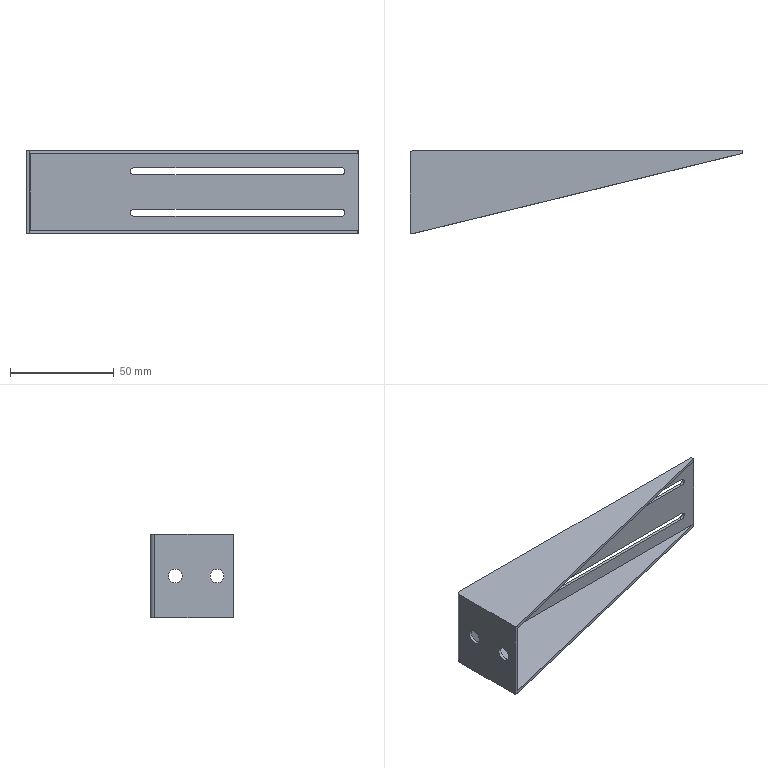Part | NX | 1 solid | 24 faces | box 160 x 40 x 40 mm | volume 19881 mm3 | plane 16 | cylinder 8 | commonest cylinder face diameters 3.4 x4 6.6 x2 1 x1 4 x1
STEP:
#1=CARTESIAN_POINT('',(159.99,-1.5,-18.5));
#2=VERTEX_POINT('',#1);
#3=CARTESIAN_POINT('',(2.,-1.5,-18.5));
#4=VERTEX_POINT('',#3);
#5=CARTESIAN_POINT('',(0.,-1.5,-18.5));
#6=DIRECTION('',(-1.,0.,0.));
#7=VECTOR('',#6,1000.);
#8=LINE('',#5,#7);
#9=EDGE_CURVE('',#2,#4,#8,.T.);
#10=ORIENTED_EDGE('',*,*,#9,.F.);
#11=CARTESIAN_POINT('',(159.99,-1.5,-20.));
#12=VERTEX_POINT('',#11);
#13=CARTESIAN_POINT('',(159.99,-1.5,20.));
#14=DIRECTION('',(0.,0.,1.));
#15=VECTOR('',#14,1000.);
#16=LINE('',#13,#15);
#17=EDGE_CURVE('',#2,#12,#16,.F.);
#18=ORIENTED_EDGE('',*,*,#17,.T.);
#19=CARTESIAN_POINT('',(160.,-1.5,-20.));
#20=VERTEX_POINT('',#19);
#21=CARTESIAN_POINT('',(0.,-1.5,-20.));
#22=DIRECTION('',(1.,0.,0.));
#23=VECTOR('',#22,1000.);
#24=LINE('',#21,#23);
#25=EDGE_CURVE('',#12,#20,#24,.T.);
#26=ORIENTED_EDGE('',*,*,#25,.T.);
#27=CARTESIAN_POINT('',(160.,-1.5,20.));
#28=VERTEX_POINT('',#27);
#29=CARTESIAN_POINT('',(160.,-1.5,20.));
#30=DIRECTION('',(0.,0.,-1.));
#31=VECTOR('',#30,1000.);
#32=LINE('',#29,#31);
#33=EDGE_CURVE('',#28,#20,#32,.T.);
#34=ORIENTED_EDGE('',*,*,#33,.F.);
#35=CARTESIAN_POINT('',(159.99,-1.5,20.));
#36=VERTEX_POINT('',#35);
#37=CARTESIAN_POINT('',(0.,-1.5,20.));
#38=DIRECTION('',(1.,0.,0.));
#39=VECTOR('',#38,1000.);
#40=LINE('',#37,#39);
#41=EDGE_CURVE('',#36,#28,#40,.T.);
#42=ORIENTED_EDGE('',*,*,#41,.F.);
#43=CARTESIAN_POINT('',(159.99,-1.5,18.5));
#44=VERTEX_POINT('',#43);
#45=CARTESIAN_POINT('',(159.99,-1.5,20.));
#46=DIRECTION('',(0.,0.,-1.));
#47=VECTOR('',#46,1000.);
#48=LINE('',#45,#47);
#49=EDGE_CURVE('',#36,#44,#48,.T.);
#50=ORIENTED_EDGE('',*,*,#49,.T.);
#51=CARTESIAN_POINT('',(2.,-1.5,18.5));
#52=VERTEX_POINT('',#51);
#53=CARTESIAN_POINT('',(0.,-1.5,18.5));
#54=DIRECTION('',(1.,0.,0.));
#55=VECTOR('',#54,1000.);
#56=LINE('',#53,#55);
#57=EDGE_CURVE('',#52,#44,#56,.T.);
#58=ORIENTED_EDGE('',*,*,#57,.F.);
#59=CARTESIAN_POINT('',(2.,-1.5,20.));
#60=DIRECTION('',(0.,0.,-1.));
#61=VECTOR('',#60,1000.);
#62=LINE('',#59,#61);
#63=EDGE_CURVE('',#52,#4,#62,.T.);
#64=ORIENTED_EDGE('',*,*,#63,.T.);
#65=EDGE_LOOP('',(#10,#18,#26,#34,#42,#50,#58,#64));
#66=FACE_BOUND('',#65,.T.);
#67=CARTESIAN_POINT('',(152.,-1.5,8.3));
#68=VERTEX_POINT('',#67);
#69=CARTESIAN_POINT('',(52.,-1.5,8.3));
#70=VERTEX_POINT('',#69);
#71=CARTESIAN_POINT('',(52.,-1.5,8.3));
#72=DIRECTION('',(-1.,0.,0.));
#73=VECTOR('',#72,1000.);
#74=LINE('',#71,#73);
#75=EDGE_CURVE('',#68,#70,#74,.T.);
#76=ORIENTED_EDGE('',*,*,#75,.T.);
#77=CARTESIAN_POINT('',(52.,-1.5,11.7));
#78=VERTEX_POINT('',#77);
#79=CARTESIAN_POINT('',(52.,-1.5,10.));
#80=DIRECTION('',(0.,1.,0.));
#81=DIRECTION('',(0.,0.,1.));
#82=AXIS2_PLACEMENT_3D('',#79,#80,#81);
#83=CIRCLE('',#82,1.7);
#84=EDGE_CURVE('',#70,#78,#83,.T.);
#85=ORIENTED_EDGE('',*,*,#84,.T.);
#86=CARTESIAN_POINT('',(152.,-1.5,11.7));
#87=VERTEX_POINT('',#86);
#88=CARTESIAN_POINT('',(52.,-1.5,11.7));
#89=DIRECTION('',(1.,0.,0.));
#90=VECTOR('',#89,1000.);
#91=LINE('',#88,#90);
#92=EDGE_CURVE('',#78,#87,#91,.T.);
#93=ORIENTED_EDGE('',*,*,#92,.T.);
#94=CARTESIAN_POINT('',(152.,-1.5,10.));
#95=DIRECTION('',(0.,1.,0.));
#96=DIRECTION('',(0.,0.,1.));
#97=AXIS2_PLACEMENT_3D('',#94,#95,#96);
#98=CIRCLE('',#97,1.7);
#99=EDGE_CURVE('',#87,#68,#98,.T.);
#100=ORIENTED_EDGE('',*,*,#99,.T.);
#101=EDGE_LOOP('',(#76,#85,#93,#100));
#102=FACE_BOUND('',#101,.T.);
#103=CARTESIAN_POINT('',(52.,-1.5,-8.3));
#104=VERTEX_POINT('',#103);
#105=CARTESIAN_POINT('',(52.,-1.5,-11.7));
#106=VERTEX_POINT('',#105);
#107=CARTESIAN_POINT('',(52.,-1.5,-10.));
#108=DIRECTION('',(0.,-1.,0.));
#109=DIRECTION('',(0.,0.,-1.));
#110=AXIS2_PLACEMENT_3D('',#107,#108,#109);
#111=CIRCLE('',#110,1.7);
#112=EDGE_CURVE('',#104,#106,#111,.T.);
#113=ORIENTED_EDGE('',*,*,#112,.F.);
#114=CARTESIAN_POINT('',(152.,-1.5,-8.3));
#115=VERTEX_POINT('',#114);
#116=CARTESIAN_POINT('',(52.,-1.5,-8.3));
#117=DIRECTION('',(-1.,0.,0.));
#118=VECTOR('',#117,1000.);
#119=LINE('',#116,#118);
#120=EDGE_CURVE('',#115,#104,#119,.T.);
#121=ORIENTED_EDGE('',*,*,#120,.F.);
#122=CARTESIAN_POINT('',(152.,-1.5,-11.7));
#123=VERTEX_POINT('',#122);
#124=CARTESIAN_POINT('',(152.,-1.5,-10.));
#125=DIRECTION('',(0.,-1.,0.));
#126=DIRECTION('',(0.,0.,-1.));
#127=AXIS2_PLACEMENT_3D('',#124,#125,#126);
#128=CIRCLE('',#127,1.7);
#129=EDGE_CURVE('',#123,#115,#128,.T.);
#130=ORIENTED_EDGE('',*,*,#129,.F.);
#131=CARTESIAN_POINT('',(52.,-1.5,-11.7));
#132=DIRECTION('',(1.,0.,0.));
#133=VECTOR('',#132,1000.);
#134=LINE('',#131,#133);
#135=EDGE_CURVE('',#106,#123,#134,.T.);
#136=ORIENTED_EDGE('',*,*,#135,.F.);
#137=EDGE_LOOP('',(#113,#121,#130,#136));
#138=FACE_BOUND('',#137,.T.);
#139=CARTESIAN_POINT('',(0.,-1.5,20.));
#140=DIRECTION('',(0.,1.,0.));
#141=DIRECTION('',(0.,0.,1.));
#142=AXIS2_PLACEMENT_3D('',#139,#140,#141);
#143=PLANE('',#142);
#144=ADVANCED_FACE('',(#66,#102,#138),#143,.F.);
#145=CARTESIAN_POINT('',(52.,0.,8.3));
#146=VERTEX_POINT('',#145);
#147=CARTESIAN_POINT('',(52.,0.,11.7));
#148=VERTEX_POINT('',#147);
#149=CARTESIAN_POINT('',(52.,0.,10.));
#150=DIRECTION('',(0.,1.,0.));
#151=DIRECTION('',(0.,0.,1.));
#152=AXIS2_PLACEMENT_3D('',#149,#150,#151);
#153=CIRCLE('',#152,1.7);
#154=EDGE_CURVE('',#146,#148,#153,.T.);
#155=ORIENTED_EDGE('',*,*,#154,.F.);
#156=CARTESIAN_POINT('',(152.,0.,8.3));
#157=VERTEX_POINT('',#156);
#158=CARTESIAN_POINT('',(52.,0.,8.3));
#159=DIRECTION('',(-1.,0.,0.));
#160=VECTOR('',#159,1000.);
#161=LINE('',#158,#160);
#162=EDGE_CURVE('',#157,#146,#161,.T.);
#163=ORIENTED_EDGE('',*,*,#162,.F.);
#164=CARTESIAN_POINT('',(152.,0.,11.7));
#165=VERTEX_POINT('',#164);
#166=CARTESIAN_POINT('',(152.,0.,10.));
#167=DIRECTION('',(0.,1.,0.));
#168=DIRECTION('',(0.,0.,1.));
#169=AXIS2_PLACEMENT_3D('',#166,#167,#168);
#170=CIRCLE('',#169,1.7);
#171=EDGE_CURVE('',#165,#157,#170,.T.);
#172=ORIENTED_EDGE('',*,*,#171,.F.);
#173=CARTESIAN_POINT('',(52.,0.,11.7));
#174=DIRECTION('',(1.,0.,0.));
#175=VECTOR('',#174,1000.);
#176=LINE('',#173,#175);
#177=EDGE_CURVE('',#148,#165,#176,.T.);
#178=ORIENTED_EDGE('',*,*,#177,.F.);
#179=EDGE_LOOP('',(#155,#163,#172,#178));
#180=FACE_BOUND('',#179,.T.);
#181=CARTESIAN_POINT('',(2.,0.,-20.));
#182=VERTEX_POINT('',#181);
#183=CARTESIAN_POINT('',(160.,0.,-20.));
#184=VERTEX_POINT('',#183);
#185=CARTESIAN_POINT('',(0.,0.,-20.));
#186=DIRECTION('',(1.,0.,0.));
#187=VECTOR('',#186,1000.);
#188=LINE('',#185,#187);
#189=EDGE_CURVE('',#182,#184,#188,.T.);
#190=ORIENTED_EDGE('',*,*,#189,.F.);
#191=CARTESIAN_POINT('',(2.,0.,20.));
#192=VERTEX_POINT('',#191);
#193=CARTESIAN_POINT('',(2.,0.,20.));
#194=DIRECTION('',(0.,0.,-1.));
#195=VECTOR('',#194,1000.);
#196=LINE('',#193,#195);
#197=EDGE_CURVE('',#192,#182,#196,.T.);
#198=ORIENTED_EDGE('',*,*,#197,.F.);
#199=CARTESIAN_POINT('',(160.,0.,20.));
#200=VERTEX_POINT('',#199);
#201=CARTESIAN_POINT('',(0.,0.,20.));
#202=DIRECTION('',(1.,0.,0.));
#203=VECTOR('',#202,1000.);
#204=LINE('',#201,#203);
#205=EDGE_CURVE('',#192,#200,#204,.T.);
#206=ORIENTED_EDGE('',*,*,#205,.T.);
#207=CARTESIAN_POINT('',(160.,0.,20.));
#208=DIRECTION('',(0.,0.,-1.));
#209=VECTOR('',#208,1000.);
#210=LINE('',#207,#209);
#211=EDGE_CURVE('',#200,#184,#210,.T.);
#212=ORIENTED_EDGE('',*,*,#211,.T.);
#213=EDGE_LOOP('',(#190,#198,#206,#212));
#214=FACE_BOUND('',#213,.T.);
#215=CARTESIAN_POINT('',(152.,0.,-8.3));
#216=VERTEX_POINT('',#215);
#217=CARTESIAN_POINT('',(52.,0.,-8.3));
#218=VERTEX_POINT('',#217);
#219=CARTESIAN_POINT('',(52.,0.,-8.3));
#220=DIRECTION('',(-1.,0.,0.));
#221=VECTOR('',#220,1000.);
#222=LINE('',#219,#221);
#223=EDGE_CURVE('',#216,#218,#222,.T.);
#224=ORIENTED_EDGE('',*,*,#223,.T.);
#225=CARTESIAN_POINT('',(52.,0.,-11.7));
#226=VERTEX_POINT('',#225);
#227=CARTESIAN_POINT('',(52.,0.,-10.));
#228=DIRECTION('',(0.,-1.,0.));
#229=DIRECTION('',(0.,0.,-1.));
#230=AXIS2_PLACEMENT_3D('',#227,#228,#229);
#231=CIRCLE('',#230,1.7);
#232=EDGE_CURVE('',#218,#226,#231,.T.);
#233=ORIENTED_EDGE('',*,*,#232,.T.);
#234=CARTESIAN_POINT('',(152.,0.,-11.7));
#235=VERTEX_POINT('',#234);
#236=CARTESIAN_POINT('',(52.,0.,-11.7));
#237=DIRECTION('',(1.,0.,0.));
#238=VECTOR('',#237,1000.);
#239=LINE('',#236,#238);
#240=EDGE_CURVE('',#226,#235,#239,.T.);
#241=ORIENTED_EDGE('',*,*,#240,.T.);
#242=CARTESIAN_POINT('',(152.,0.,-10.));
#243=DIRECTION('',(0.,-1.,0.));
#244=DIRECTION('',(0.,0.,-1.));
#245=AXIS2_PLACEMENT_3D('',#242,#243,#244);
#246=CIRCLE('',#245,1.7);
#247=EDGE_CURVE('',#235,#216,#246,.T.);
#248=ORIENTED_EDGE('',*,*,#247,.T.);
#249=EDGE_LOOP('',(#224,#233,#241,#248));
#250=FACE_BOUND('',#249,.T.);
#251=CARTESIAN_POINT('',(0.,0.,20.));
#252=DIRECTION('',(0.,1.,0.));
#253=DIRECTION('',(0.,0.,1.));
#254=AXIS2_PLACEMENT_3D('',#251,#252,#253);
#255=PLANE('',#254);
#256=ADVANCED_FACE('',(#180,#214,#250),#255,.T.);
#257=CARTESIAN_POINT('',(1.5,-12.,3.3));
#258=VERTEX_POINT('',#257);
#259=CARTESIAN_POINT('',(1.5,-12.,0.));
#260=DIRECTION('',(-1.,0.,0.));
#261=DIRECTION('',(0.,0.,1.));
#262=AXIS2_PLACEMENT_3D('',#259,#260,#261);
#263=CIRCLE('',#262,3.3);
#264=EDGE_CURVE('',#258,#258,#263,.T.);
#265=ORIENTED_EDGE('',*,*,#264,.T.);
#266=EDGE_LOOP('',(#265));
#267=FACE_BOUND('',#266,.T.);
#268=CARTESIAN_POINT('',(1.5,-32.,3.3));
#269=VERTEX_POINT('',#268);
#270=CARTESIAN_POINT('',(1.5,-32.,0.));
#271=DIRECTION('',(-1.,0.,0.));
#272=DIRECTION('',(0.,0.,1.));
#273=AXIS2_PLACEMENT_3D('',#270,#271,#272);
#274=CIRCLE('',#273,3.3);
#275=EDGE_CURVE('',#269,#269,#274,.T.);
#276=ORIENTED_EDGE('',*,*,#275,.T.);
#277=EDGE_LOOP('',(#276));
#278=FACE_BOUND('',#277,.T.);
#279=CARTESIAN_POINT('',(1.5,-2.,-18.5));
#280=VERTEX_POINT('',#279);
#281=CARTESIAN_POINT('',(1.5,-40.,-18.5));
#282=VERTEX_POINT('',#281);
#283=CARTESIAN_POINT('',(1.5,-40.,-18.5));
#284=DIRECTION('',(0.,-1.,0.));
#285=VECTOR('',#284,1000.);
#286=LINE('',#283,#285);
#287=EDGE_CURVE('',#280,#282,#286,.T.);
#288=ORIENTED_EDGE('',*,*,#287,.F.);
#289=CARTESIAN_POINT('',(1.5,-2.,18.5));
#290=VERTEX_POINT('',#289);
#291=CARTESIAN_POINT('',(1.5,-2.,20.));
#292=DIRECTION('',(0.,0.,-1.));
#293=VECTOR('',#292,1000.);
#294=LINE('',#291,#293);
#295=EDGE_CURVE('',#290,#280,#294,.T.);
#296=ORIENTED_EDGE('',*,*,#295,.F.);
#297=CARTESIAN_POINT('',(1.5,-40.,18.5));
#298=VERTEX_POINT('',#297);
#299=CARTESIAN_POINT('',(1.5,-40.,18.5));
#300=DIRECTION('',(0.,1.,0.));
#301=VECTOR('',#300,1000.);
#302=LINE('',#299,#301);
#303=EDGE_CURVE('',#298,#290,#302,.T.);
#304=ORIENTED_EDGE('',*,*,#303,.F.);
#305=CARTESIAN_POINT('',(1.5,-40.,20.));
#306=DIRECTION('',(0.,0.,-1.));
#307=VECTOR('',#306,1000.);
#308=LINE('',#305,#307);
#309=EDGE_CURVE('',#298,#282,#308,.T.);
#310=ORIENTED_EDGE('',*,*,#309,.T.);
#311=EDGE_LOOP('',(#288,#296,#304,#310));
#312=FACE_BOUND('',#311,.T.);
#313=CARTESIAN_POINT('',(1.5,-40.,20.));
#314=DIRECTION('',(-1.,0.,0.));
#315=DIRECTION('',(0.,0.,1.));
#316=AXIS2_PLACEMENT_3D('',#313,#314,#315);
#317=PLANE('',#316);
#318=ADVANCED_FACE('',(#267,#278,#312),#317,.F.);
#319=CARTESIAN_POINT('',(2.,-2.,-18.5));
#320=DIRECTION('',(0.,0.,-1.));
#321=DIRECTION('',(-1.,0.,0.));
#322=AXIS2_PLACEMENT_3D('',#319,#320,#321);
#323=CIRCLE('',#322,0.5);
#324=EDGE_CURVE('',#4,#280,#323,.F.);
#325=ORIENTED_EDGE('',*,*,#324,.F.);
#326=ORIENTED_EDGE('',*,*,#63,.F.);
#327=CARTESIAN_POINT('',(2.,-2.,18.5));
#328=DIRECTION('',(0.,0.,1.));
#329=DIRECTION('',(1.,0.,0.));
#330=AXIS2_PLACEMENT_3D('',#327,#328,#329);
#331=CIRCLE('',#330,0.5);
#332=EDGE_CURVE('',#290,#52,#331,.F.);
#333=ORIENTED_EDGE('',*,*,#332,.F.);
#334=ORIENTED_EDGE('',*,*,#295,.T.);
#335=EDGE_LOOP('',(#325,#326,#333,#334));
#336=FACE_BOUND('',#335,.T.);
#337=CARTESIAN_POINT('',(2.,-2.,20.));
#338=DIRECTION('',(0.,0.,-1.));
#339=DIRECTION('',(-1.,0.,0.));
#340=AXIS2_PLACEMENT_3D('',#337,#338,#339);
#341=CYLINDRICAL_SURFACE('',#340,0.5);
#342=ADVANCED_FACE('',(#336),#341,.F.);
#343=ORIENTED_EDGE('',*,*,#33,.T.);
#344=CARTESIAN_POINT('',(160.,0.,-20.));
#345=DIRECTION('',(0.,-1.,0.));
#346=VECTOR('',#345,1000.);
#347=LINE('',#344,#346);
#348=EDGE_CURVE('',#184,#20,#347,.T.);
#349=ORIENTED_EDGE('',*,*,#348,.F.);
#350=ORIENTED_EDGE('',*,*,#211,.F.);
#351=CARTESIAN_POINT('',(160.,0.,20.));
#352=DIRECTION('',(0.,-1.,0.));
#353=VECTOR('',#352,1000.);
#354=LINE('',#351,#353);
#355=EDGE_CURVE('',#200,#28,#354,.T.);
#356=ORIENTED_EDGE('',*,*,#355,.T.);
#357=EDGE_LOOP('',(#343,#349,#350,#356));
#358=FACE_BOUND('',#357,.T.);
#359=CARTESIAN_POINT('',(160.,0.,20.));
#360=DIRECTION('',(1.,0.,0.));
#361=DIRECTION('',(0.,0.,-1.));
#362=AXIS2_PLACEMENT_3D('',#359,#360,#361);
#363=PLANE('',#362);
#364=ADVANCED_FACE('',(#358),#363,.T.);
#365=CARTESIAN_POINT('',(0.,-2.,-20.));
#366=VERTEX_POINT('',#365);
#367=CARTESIAN_POINT('',(2.,-2.,-20.));
#368=DIRECTION('',(0.,0.,1.));
#369=DIRECTION('',(1.,0.,0.));
#370=AXIS2_PLACEMENT_3D('',#367,#368,#369);
#371=CIRCLE('',#370,2.);
#372=EDGE_CURVE('',#366,#182,#371,.F.);
#373=ORIENTED_EDGE('',*,*,#372,.F.);
#374=CARTESIAN_POINT('',(0.,-2.,20.));
#375=VERTEX_POINT('',#374);
#376=CARTESIAN_POINT('',(0.,-2.,20.));
#377=DIRECTION('',(0.,0.,-1.));
#378=VECTOR('',#377,1000.);
#379=LINE('',#376,#378);
#380=EDGE_CURVE('',#375,#366,#379,.T.);
#381=ORIENTED_EDGE('',*,*,#380,.F.);
#382=CARTESIAN_POINT('',(2.,-2.,20.));
#383=DIRECTION('',(0.,0.,1.));
#384=DIRECTION('',(1.,0.,0.));
#385=AXIS2_PLACEMENT_3D('',#382,#383,#384);
#386=CIRCLE('',#385,2.);
#387=EDGE_CURVE('',#375,#192,#386,.F.);
#388=ORIENTED_EDGE('',*,*,#387,.T.);
#389=ORIENTED_EDGE('',*,*,#197,.T.);
#390=EDGE_LOOP('',(#373,#381,#388,#389));
#391=FACE_BOUND('',#390,.T.);
#392=CARTESIAN_POINT('',(2.,-2.,20.));
#393=DIRECTION('',(0.,0.,-1.));
#394=DIRECTION('',(-1.,0.,0.));
#395=AXIS2_PLACEMENT_3D('',#392,#393,#394);
#396=CYLINDRICAL_SURFACE('',#395,2.);
#397=ADVANCED_FACE('',(#391),#396,.T.);
#398=CARTESIAN_POINT('',(0.,-12.,3.3));
#399=VERTEX_POINT('',#398);
#400=CARTESIAN_POINT('',(0.,-12.,0.));
#401=DIRECTION('',(-1.,0.,0.));
#402=DIRECTION('',(0.,0.,1.));
#403=AXIS2_PLACEMENT_3D('',#400,#401,#402);
#404=CIRCLE('',#403,3.3);
#405=EDGE_CURVE('',#399,#399,#404,.T.);
#406=ORIENTED_EDGE('',*,*,#405,.F.);
#407=EDGE_LOOP('',(#406));
#408=FACE_BOUND('',#407,.T.);
#409=CARTESIAN_POINT('',(0.,-32.,3.3));
#410=VERTEX_POINT('',#409);
#411=CARTESIAN_POINT('',(0.,-32.,0.));
#412=DIRECTION('',(-1.,0.,0.));
#413=DIRECTION('',(0.,0.,1.));
#414=AXIS2_PLACEMENT_3D('',#411,#412,#413);
#415=CIRCLE('',#414,3.3);
#416=EDGE_CURVE('',#410,#410,#415,.T.);
#417=ORIENTED_EDGE('',*,*,#416,.F.);
#418=EDGE_LOOP('',(#417));
#419=FACE_BOUND('',#418,.T.);
#420=CARTESIAN_POINT('',(0.,-40.,-20.));
#421=VERTEX_POINT('',#420);
#422=CARTESIAN_POINT('',(0.,-40.,-20.));
#423=DIRECTION('',(0.,1.,0.));
#424=VECTOR('',#423,1000.);
#425=LINE('',#422,#424);
#426=EDGE_CURVE('',#421,#366,#425,.T.);
#427=ORIENTED_EDGE('',*,*,#426,.F.);
#428=CARTESIAN_POINT('',(0.,-40.,20.));
#429=VERTEX_POINT('',#428);
#430=CARTESIAN_POINT('',(0.,-40.,20.));
#431=DIRECTION('',(0.,0.,-1.));
#432=VECTOR('',#431,1000.);
#433=LINE('',#430,#432);
#434=EDGE_CURVE('',#429,#421,#433,.T.);
#435=ORIENTED_EDGE('',*,*,#434,.F.);
#436=CARTESIAN_POINT('',(0.,-40.,20.));
#437=DIRECTION('',(0.,1.,0.));
#438=VECTOR('',#437,1000.);
#439=LINE('',#436,#438);
#440=EDGE_CURVE('',#429,#375,#439,.T.);
#441=ORIENTED_EDGE('',*,*,#440,.T.);
#442=ORIENTED_EDGE('',*,*,#380,.T.);
#443=EDGE_LOOP('',(#427,#435,#441,#442));
#444=FACE_BOUND('',#443,.T.);
#445=CARTESIAN_POINT('',(0.,-40.,20.));
#446=DIRECTION('',(-1.,0.,0.));
#447=DIRECTION('',(0.,0.,1.));
#448=AXIS2_PLACEMENT_3D('',#445,#446,#447);
#449=PLANE('',#448);
#450=ADVANCED_FACE('',(#408,#419,#444),#449,.T.);
#451=CARTESIAN_POINT('',(1.5,-40.,-20.));
#452=VERTEX_POINT('',#451);
#453=CARTESIAN_POINT('',(1.5,-40.,20.));
#454=DIRECTION('',(0.,0.,-1.));
#455=VECTOR('',#454,1000.);
#456=LINE('',#453,#455);
#457=EDGE_CURVE('',#452,#282,#456,.F.);
#458=ORIENTED_EDGE('',*,*,#457,.T.);
#459=ORIENTED_EDGE('',*,*,#309,.F.);
#460=CARTESIAN_POINT('',(1.5,-40.,20.));
#461=VERTEX_POINT('',#460);
#462=CARTESIAN_POINT('',(1.5,-40.,20.));
#463=DIRECTION('',(0.,0.,-1.));
#464=VECTOR('',#463,1000.);
#465=LINE('',#462,#464);
#466=EDGE_CURVE('',#461,#298,#465,.T.);
#467=ORIENTED_EDGE('',*,*,#466,.F.);
#468=CARTESIAN_POINT('',(1.5,-40.,20.));
#469=DIRECTION('',(-1.,0.,0.));
#470=VECTOR('',#469,1000.);
#471=LINE('',#468,#470);
#472=EDGE_CURVE('',#461,#429,#471,.T.);
#473=ORIENTED_EDGE('',*,*,#472,.T.);
#474=ORIENTED_EDGE('',*,*,#434,.T.);
#475=CARTESIAN_POINT('',(1.5,-40.,-20.));
#476=DIRECTION('',(-1.,0.,0.));
#477=VECTOR('',#476,1000.);
#478=LINE('',#475,#477);
#479=EDGE_CURVE('',#452,#421,#478,.T.);
#480=ORIENTED_EDGE('',*,*,#479,.F.);
#481=EDGE_LOOP('',(#458,#459,#467,#473,#474,#480));
#482=FACE_BOUND('',#481,.T.);
#483=CARTESIAN_POINT('',(1.5,-40.,20.));
#484=DIRECTION('',(0.,-1.,0.));
#485=DIRECTION('',(0.,0.,-1.));
#486=AXIS2_PLACEMENT_3D('',#483,#484,#485);
#487=PLANE('',#486);
#488=ADVANCED_FACE('',(#482),#487,.T.);
#489=CARTESIAN_POINT('',(1.5,-40.,20.));
#490=DIRECTION('',(0.9717,0.2361,0.));
#491=VECTOR('',#490,1000.);
#492=LINE('',#489,#491);
#493=EDGE_CURVE('',#461,#36,#492,.T.);
#494=ORIENTED_EDGE('',*,*,#493,.T.);
#495=ORIENTED_EDGE('',*,*,#41,.T.);
#496=ORIENTED_EDGE('',*,*,#355,.F.);
#497=ORIENTED_EDGE('',*,*,#205,.F.);
#498=ORIENTED_EDGE('',*,*,#387,.F.);
#499=ORIENTED_EDGE('',*,*,#440,.F.);
#500=ORIENTED_EDGE('',*,*,#472,.F.);
#501=EDGE_LOOP('',(#494,#495,#496,#497,#498,#499,#500));
#502=FACE_BOUND('',#501,.T.);
#503=CARTESIAN_POINT('',(2.,-2.,20.));
#504=DIRECTION('',(0.,0.,1.));
#505=DIRECTION('',(1.,0.,0.));
#506=AXIS2_PLACEMENT_3D('',#503,#504,#505);
#507=PLANE('',#506);
#508=ADVANCED_FACE('',(#502),#507,.T.);
#509=ORIENTED_EDGE('',*,*,#25,.F.);
#510=CARTESIAN_POINT('',(1.5,-40.,-20.));
#511=DIRECTION('',(0.9717,0.2361,0.));
#512=VECTOR('',#511,1000.);
#513=LINE('',#510,#512);
#514=EDGE_CURVE('',#452,#12,#513,.T.);
#515=ORIENTED_EDGE('',*,*,#514,.F.);
#516=ORIENTED_EDGE('',*,*,#479,.T.);
#517=ORIENTED_EDGE('',*,*,#426,.T.);
#518=ORIENTED_EDGE('',*,*,#372,.T.);
#519=ORIENTED_EDGE('',*,*,#189,.T.);
#520=ORIENTED_EDGE('',*,*,#348,.T.);
#521=EDGE_LOOP('',(#509,#515,#516,#517,#518,#519,#520));
#522=FACE_BOUND('',#521,.T.);
#523=CARTESIAN_POINT('',(2.,-2.,-20.));
#524=DIRECTION('',(0.,0.,1.));
#525=DIRECTION('',(1.,0.,0.));
#526=AXIS2_PLACEMENT_3D('',#523,#524,#525);
#527=PLANE('',#526);
#528=ADVANCED_FACE('',(#522),#527,.F.);
#529=ORIENTED_EDGE('',*,*,#49,.F.);
#530=ORIENTED_EDGE('',*,*,#493,.F.);
#531=ORIENTED_EDGE('',*,*,#466,.T.);
#532=CARTESIAN_POINT('',(1.5,-40.,18.5));
#533=DIRECTION('',(0.9717,0.2361,0.));
#534=VECTOR('',#533,1000.);
#535=LINE('',#532,#534);
#536=EDGE_CURVE('',#298,#44,#535,.T.);
#537=ORIENTED_EDGE('',*,*,#536,.T.);
#538=EDGE_LOOP('',(#529,#530,#531,#537));
#539=FACE_BOUND('',#538,.T.);
#540=CARTESIAN_POINT('',(1.5,-40.,20.));
#541=DIRECTION('',(0.2361,-0.9717,0.));
#542=DIRECTION('',(0.9717,0.2361,0.));
#543=AXIS2_PLACEMENT_3D('',#540,#541,#542);
#544=PLANE('',#543);
#545=ADVANCED_FACE('',(#539),#544,.T.);
#546=ORIENTED_EDGE('',*,*,#332,.T.);
#547=ORIENTED_EDGE('',*,*,#57,.T.);
#548=ORIENTED_EDGE('',*,*,#536,.F.);
#549=ORIENTED_EDGE('',*,*,#303,.T.);
#550=EDGE_LOOP('',(#546,#547,#548,#549));
#551=FACE_BOUND('',#550,.T.);
#552=CARTESIAN_POINT('',(80.,-20.,18.5));
#553=DIRECTION('',(0.,0.,1.));
#554=DIRECTION('',(1.,0.,0.));
#555=AXIS2_PLACEMENT_3D('',#552,#553,#554);
#556=PLANE('',#555);
#557=ADVANCED_FACE('',(#551),#556,.F.);
#558=ORIENTED_EDGE('',*,*,#154,.T.);
#559=CARTESIAN_POINT('',(52.,-1.5,11.7));
#560=DIRECTION('',(0.,1.,0.));
#561=VECTOR('',#560,1000.);
#562=LINE('',#559,#561);
#563=EDGE_CURVE('',#78,#148,#562,.T.);
#564=ORIENTED_EDGE('',*,*,#563,.F.);
#565=ORIENTED_EDGE('',*,*,#84,.F.);
#566=CARTESIAN_POINT('',(52.,-1.5,8.3));
#567=DIRECTION('',(0.,1.,0.));
#568=VECTOR('',#567,1000.);
#569=LINE('',#566,#568);
#570=EDGE_CURVE('',#70,#146,#569,.T.);
#571=ORIENTED_EDGE('',*,*,#570,.T.);
#572=EDGE_LOOP('',(#558,#564,#565,#571));
#573=FACE_BOUND('',#572,.T.);
#574=CARTESIAN_POINT('',(52.,-1.5,10.));
#575=DIRECTION('',(0.,1.,0.));
#576=DIRECTION('',(0.,0.,1.));
#577=AXIS2_PLACEMENT_3D('',#574,#575,#576);
#578=CYLINDRICAL_SURFACE('',#577,1.7);
#579=ADVANCED_FACE('',(#573),#578,.F.);
#580=ORIENTED_EDGE('',*,*,#162,.T.);
#581=ORIENTED_EDGE('',*,*,#570,.F.);
#582=ORIENTED_EDGE('',*,*,#75,.F.);
#583=CARTESIAN_POINT('',(152.,-1.5,8.3));
#584=DIRECTION('',(0.,1.,0.));
#585=VECTOR('',#584,1000.);
#586=LINE('',#583,#585);
#587=EDGE_CURVE('',#68,#157,#586,.T.);
#588=ORIENTED_EDGE('',*,*,#587,.T.);
#589=EDGE_LOOP('',(#580,#581,#582,#588));
#590=FACE_BOUND('',#589,.T.);
#591=CARTESIAN_POINT('',(52.,-1.5,8.3));
#592=DIRECTION('',(0.,0.,-1.));
#593=DIRECTION('',(-1.,0.,0.));
#594=AXIS2_PLACEMENT_3D('',#591,#592,#593);
#595=PLANE('',#594);
#596=ADVANCED_FACE('',(#590),#595,.F.);
#597=ORIENTED_EDGE('',*,*,#171,.T.);
#598=ORIENTED_EDGE('',*,*,#587,.F.);
#599=ORIENTED_EDGE('',*,*,#99,.F.);
#600=CARTESIAN_POINT('',(152.,-1.5,11.7));
#601=DIRECTION('',(0.,1.,0.));
#602=VECTOR('',#601,1000.);
#603=LINE('',#600,#602);
#604=EDGE_CURVE('',#87,#165,#603,.T.);
#605=ORIENTED_EDGE('',*,*,#604,.T.);
#606=EDGE_LOOP('',(#597,#598,#599,#605));
#607=FACE_BOUND('',#606,.T.);
#608=CARTESIAN_POINT('',(152.,-1.5,10.));
#609=DIRECTION('',(0.,1.,0.));
#610=DIRECTION('',(0.,0.,1.));
#611=AXIS2_PLACEMENT_3D('',#608,#609,#610);
#612=CYLINDRICAL_SURFACE('',#611,1.7);
#613=ADVANCED_FACE('',(#607),#612,.F.);
#614=ORIENTED_EDGE('',*,*,#177,.T.);
#615=ORIENTED_EDGE('',*,*,#604,.F.);
#616=ORIENTED_EDGE('',*,*,#92,.F.);
#617=ORIENTED_EDGE('',*,*,#563,.T.);
#618=EDGE_LOOP('',(#614,#615,#616,#617));
#619=FACE_BOUND('',#618,.T.);
#620=CARTESIAN_POINT('',(52.,-1.5,11.7));
#621=DIRECTION('',(0.,0.,1.));
#622=DIRECTION('',(1.,0.,0.));
#623=AXIS2_PLACEMENT_3D('',#620,#621,#622);
#624=PLANE('',#623);
#625=ADVANCED_FACE('',(#619),#624,.F.);
#626=CARTESIAN_POINT('',(1.5,-40.,-18.5));
#627=DIRECTION('',(0.9717,0.2361,0.));
#628=VECTOR('',#627,1000.);
#629=LINE('',#626,#628);
#630=EDGE_CURVE('',#282,#2,#629,.T.);
#631=ORIENTED_EDGE('',*,*,#630,.T.);
#632=ORIENTED_EDGE('',*,*,#9,.T.);
#633=ORIENTED_EDGE('',*,*,#324,.T.);
#634=ORIENTED_EDGE('',*,*,#287,.T.);
#635=EDGE_LOOP('',(#631,#632,#633,#634));
#636=FACE_BOUND('',#635,.T.);
#637=CARTESIAN_POINT('',(80.,-20.,-18.5));
#638=DIRECTION('',(0.,0.,-1.));
#639=DIRECTION('',(-1.,0.,0.));
#640=AXIS2_PLACEMENT_3D('',#637,#638,#639);
#641=PLANE('',#640);
#642=ADVANCED_FACE('',(#636),#641,.F.);
#643=ORIENTED_EDGE('',*,*,#17,.F.);
#644=ORIENTED_EDGE('',*,*,#630,.F.);
#645=ORIENTED_EDGE('',*,*,#457,.F.);
#646=ORIENTED_EDGE('',*,*,#514,.T.);
#647=EDGE_LOOP('',(#643,#644,#645,#646));
#648=FACE_BOUND('',#647,.T.);
#649=CARTESIAN_POINT('',(1.5,-40.,-20.));
#650=DIRECTION('',(-0.2361,0.9717,0.));
#651=DIRECTION('',(0.9717,0.2361,0.));
#652=AXIS2_PLACEMENT_3D('',#649,#650,#651);
#653=PLANE('',#652);
#654=ADVANCED_FACE('',(#648),#653,.F.);
#655=ORIENTED_EDGE('',*,*,#232,.F.);
#656=CARTESIAN_POINT('',(52.,-1.5,-8.3));
#657=DIRECTION('',(0.,1.,0.));
#658=VECTOR('',#657,1000.);
#659=LINE('',#656,#658);
#660=EDGE_CURVE('',#104,#218,#659,.T.);
#661=ORIENTED_EDGE('',*,*,#660,.F.);
#662=ORIENTED_EDGE('',*,*,#112,.T.);
#663=CARTESIAN_POINT('',(52.,-1.5,-11.7));
#664=DIRECTION('',(0.,1.,0.));
#665=VECTOR('',#664,1000.);
#666=LINE('',#663,#665);
#667=EDGE_CURVE('',#106,#226,#666,.T.);
#668=ORIENTED_EDGE('',*,*,#667,.T.);
#669=EDGE_LOOP('',(#655,#661,#662,#668));
#670=FACE_BOUND('',#669,.T.);
#671=CARTESIAN_POINT('',(52.,-1.5,-10.));
#672=DIRECTION('',(0.,1.,0.));
#673=DIRECTION('',(0.,0.,1.));
#674=AXIS2_PLACEMENT_3D('',#671,#672,#673);
#675=CYLINDRICAL_SURFACE('',#674,1.7);
#676=ADVANCED_FACE('',(#670),#675,.F.);
#677=ORIENTED_EDGE('',*,*,#240,.F.);
#678=ORIENTED_EDGE('',*,*,#667,.F.);
#679=ORIENTED_EDGE('',*,*,#135,.T.);
#680=CARTESIAN_POINT('',(152.,-1.5,-11.7));
#681=DIRECTION('',(0.,1.,0.));
#682=VECTOR('',#681,1000.);
#683=LINE('',#680,#682);
#684=EDGE_CURVE('',#123,#235,#683,.T.);
#685=ORIENTED_EDGE('',*,*,#684,.T.);
#686=EDGE_LOOP('',(#677,#678,#679,#685));
#687=FACE_BOUND('',#686,.T.);
#688=CARTESIAN_POINT('',(52.,-1.5,-11.7));
#689=DIRECTION('',(0.,0.,1.));
#690=DIRECTION('',(1.,0.,0.));
#691=AXIS2_PLACEMENT_3D('',#688,#689,#690);
#692=PLANE('',#691);
#693=ADVANCED_FACE('',(#687),#692,.T.);
#694=ORIENTED_EDGE('',*,*,#247,.F.);
#695=ORIENTED_EDGE('',*,*,#684,.F.);
#696=ORIENTED_EDGE('',*,*,#129,.T.);
#697=CARTESIAN_POINT('',(152.,-1.5,-8.3));
#698=DIRECTION('',(0.,1.,0.));
#699=VECTOR('',#698,1000.);
#700=LINE('',#697,#699);
#701=EDGE_CURVE('',#115,#216,#700,.T.);
#702=ORIENTED_EDGE('',*,*,#701,.T.);
#703=EDGE_LOOP('',(#694,#695,#696,#702));
#704=FACE_BOUND('',#703,.T.);
#705=CARTESIAN_POINT('',(152.,-1.5,-10.));
#706=DIRECTION('',(0.,1.,0.));
#707=DIRECTION('',(0.,0.,1.));
#708=AXIS2_PLACEMENT_3D('',#705,#706,#707);
#709=CYLINDRICAL_SURFACE('',#708,1.7);
#710=ADVANCED_FACE('',(#704),#709,.F.);
#711=ORIENTED_EDGE('',*,*,#223,.F.);
#712=ORIENTED_EDGE('',*,*,#701,.F.);
#713=ORIENTED_EDGE('',*,*,#120,.T.);
#714=ORIENTED_EDGE('',*,*,#660,.T.);
#715=EDGE_LOOP('',(#711,#712,#713,#714));
#716=FACE_BOUND('',#715,.T.);
#717=CARTESIAN_POINT('',(52.,-1.5,-8.3));
#718=DIRECTION('',(0.,0.,-1.));
#719=DIRECTION('',(-1.,0.,0.));
#720=AXIS2_PLACEMENT_3D('',#717,#718,#719);
#721=PLANE('',#720);
#722=ADVANCED_FACE('',(#716),#721,.T.);
#723=ORIENTED_EDGE('',*,*,#416,.T.);
#724=EDGE_LOOP('',(#723));
#725=FACE_BOUND('',#724,.T.);
#726=ORIENTED_EDGE('',*,*,#275,.F.);
#727=EDGE_LOOP('',(#726));
#728=FACE_BOUND('',#727,.T.);
#729=CARTESIAN_POINT('',(0.,-32.,0.));
#730=DIRECTION('',(-1.,0.,0.));
#731=DIRECTION('',(0.,0.,1.));
#732=AXIS2_PLACEMENT_3D('',#729,#730,#731);
#733=CYLINDRICAL_SURFACE('',#732,3.3);
#734=ADVANCED_FACE('',(#725,#728),#733,.F.);
#735=ORIENTED_EDGE('',*,*,#405,.T.);
#736=EDGE_LOOP('',(#735));
#737=FACE_BOUND('',#736,.T.);
#738=ORIENTED_EDGE('',*,*,#264,.F.);
#739=EDGE_LOOP('',(#738));
#740=FACE_BOUND('',#739,.T.);
#741=CARTESIAN_POINT('',(0.,-12.,0.));
#742=DIRECTION('',(-1.,0.,0.));
#743=DIRECTION('',(0.,0.,1.));
#744=AXIS2_PLACEMENT_3D('',#741,#742,#743);
#745=CYLINDRICAL_SURFACE('',#744,3.3);
#746=ADVANCED_FACE('',(#737,#740),#745,.F.);
#747=CLOSED_SHELL('',(#144,#256,#318,#342,#364,#397,#450,#488,#508,#528,#545,#557,#579,#596,#613,#625,#642,#654,#676,#693,#710,#722,#734,#746));
#748=MANIFOLD_SOLID_BREP('',#747);
#749=(LENGTH_UNIT()NAMED_UNIT(*)SI_UNIT(.MILLI.,.METRE.));
#750=UNCERTAINTY_MEASURE_WITH_UNIT(LENGTH_MEASURE(0.00001),#749,'','');
#751=(NAMED_UNIT(*)PLANE_ANGLE_UNIT()SI_UNIT($,.RADIAN.));
#752=(NAMED_UNIT(*)SI_UNIT($,.STERADIAN.)SOLID_ANGLE_UNIT());
#753=(GEOMETRIC_REPRESENTATION_CONTEXT(3)GLOBAL_UNCERTAINTY_ASSIGNED_CONTEXT((#750))GLOBAL_UNIT_ASSIGNED_CONTEXT((#749,#751,#752))REPRESENTATION_CONTEXT('',''));
#754=ADVANCED_BREP_SHAPE_REPRESENTATION('',(#748),#753);